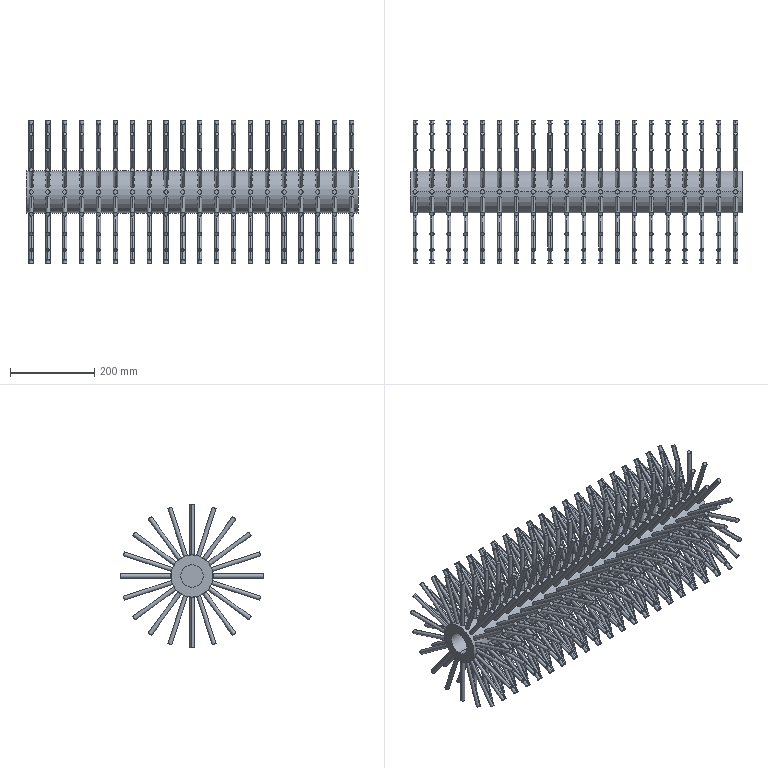Part | SolidWorks | features AEMSimFeature 1 | 401 solids | 1610 faces | box 787.42 x 340 x 340 mm | volume 9693964 mm3 | cylinder 806 | plane 804 | commonest cylinder face diameters 10 x800 53 x4 100 x2